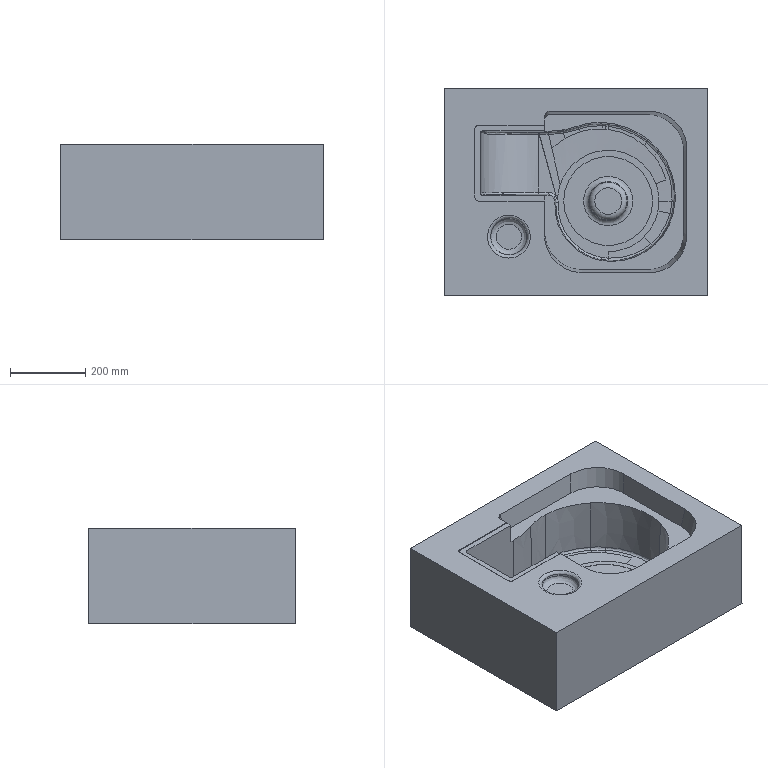CAM job | NX | 3-axis milling | part box 700 x 550 x 255 mm | stock box 700 x 550 x 255 mm
Tools:
number,name,description,diameter,corner_radius,flute_length,length,flutes
0,D50R6,Milling Tool-5 Parameters,50.0,6.0,50.0,75.0,2
0,D26R0.8,Milling Tool-5 Parameters,26.0,0.8,50.0,75.0,2
0,20,Milling Tool-5 Parameters,20.0,0.0,50.0,75.0,2
0,D8R2,Milling Tool-5 Parameters,8.0,2.0,50.0,75.0,2
Operations:
program,operation,operation_type,tool,method,geometry_group,spindle_rpm,surface_speed,feed_per_tooth,feed_cut,feed_plunge,cut_length_mm,path_length_mm,cut_time_min,machine_time_min
NC_PROGRAM,CAVITY_MILL,CavityMilling,D50R6,METHOD,WORKPIECE,1000.0,157.0,0.9,1800.0,100.0,677838.691,692305.701,376.577,378.024
NC_PROGRAM,CAVITY_MILL_COPY,CavityMilling,D50R6,METHOD,WORKPIECE,1000.0,157.0,0.9,1800.0,100.0,440942.911,452175.401,244.968,246.091
NC_PROGRAM,CAVITY_MILL_COPY_1,CavityMilling,D26R0.8,METHOD,WORKPIECE,1000.0,157.0,0.9,1800.0,100.0,104655.418,153170.543,58.142,62.993
NC_PROGRAM,ZLEVEL_PROFILE,ZLevelMilling,20,METHOD,WORKPIECE,2200.0,138.0,0.4545,2000.0,100.0,102446.239,123203.132,51.223,53.299
NC_PROGRAM,FACE_MILLING,FaceMilling,20,METHOD,WORKPIECE,0.0,0.0,0.0,250.0,100.0,3847.775,7257.41,15.391,15.732
NC_PROGRAM,FACE_MILLING_1,FaceMilling,D26R0.8,METHOD,WORKPIECE,0.0,0.0,0.0,250.0,100.0,4163.05,8326.63,16.652,17.069
NC_PROGRAM,ZLEVEL_PROFILE_COPY,ZLevelMilling,D8R2,METHOD,WORKPIECE,2600.0,65.0,0.5,2600.0,100.0,500448.347,651752.35,192.48,207.611
NC_PROGRAM,CAVITY_MILL_COPY_2,CavityMilling,D26R0.8,METHOD,WORKPIECE,2500.0,204.0,0.48,2400.0,100.0,18017.351,19600.587,7.507,7.666
NC_PROGRAM,ZLEVEL_PROFILE_1,ZLevelMilling,D26R0.8,METHOD,WORKPIECE,0.0,0.0,0.0,250.0,100.0,28010.095,29605.891,112.04,112.2